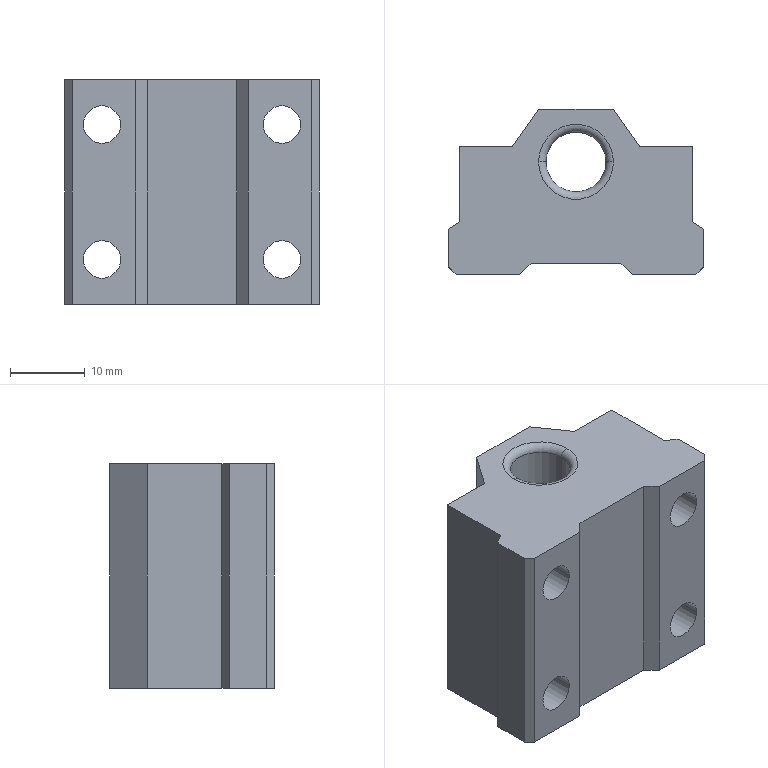Part | STEP file | Slider 8 | 1 solid | 34 faces | box 34 x 22 x 30 mm | volume 14928 mm3 | plane 20 | cylinder 10 | torus 4 | commonest cylinder face diameters 5 x8 8 x2